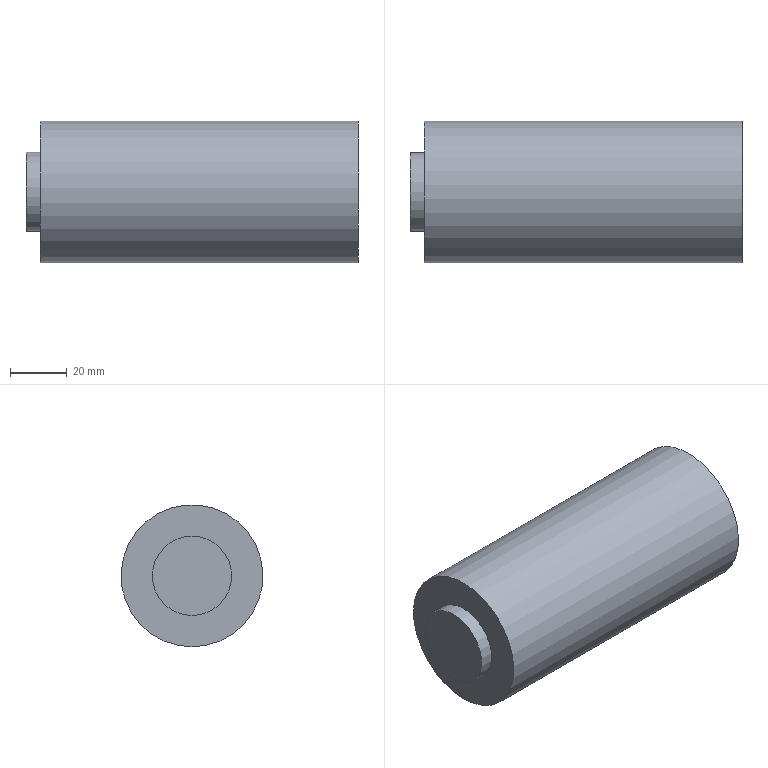Part | NX | features solid 2 | 1 solid | 5 faces | box 117 x 50 x 50 mm | volume 222990 mm3 | plane 3 | cylinder 2 | commonest cylinder face diameters 28 x1 50 x1
STEP:
#1=CARTESIAN_POINT('',(580.,930.,-200.));
#2=VERTEX_POINT('',#1);
#3=CARTESIAN_POINT('',(580.,930.,-175.));
#4=DIRECTION('',(-1.,0.,0.));
#5=DIRECTION('',(0.,0.,-1.));
#6=AXIS2_PLACEMENT_3D('',#3,#4,#5);
#7=CIRCLE('',#6,25.);
#8=EDGE_CURVE('',#2,#2,#7,.T.);
#9=ORIENTED_EDGE('',*,*,#8,.T.);
#10=EDGE_LOOP('',(#9));
#11=FACE_BOUND('',#10,.T.);
#12=CARTESIAN_POINT('',(580.,930.,-189.));
#13=VERTEX_POINT('',#12);
#14=CARTESIAN_POINT('',(580.,930.,-175.));
#15=DIRECTION('',(-1.,0.,0.));
#16=DIRECTION('',(0.,0.,-1.));
#17=AXIS2_PLACEMENT_3D('',#14,#15,#16);
#18=CIRCLE('',#17,14.);
#19=EDGE_CURVE('',#13,#13,#18,.T.);
#20=ORIENTED_EDGE('',*,*,#19,.F.);
#21=EDGE_LOOP('',(#20));
#22=FACE_BOUND('',#21,.T.);
#23=CARTESIAN_POINT('',(580.,930.,-175.));
#24=DIRECTION('',(-1.,0.,0.));
#25=DIRECTION('',(0.,0.,-1.));
#26=AXIS2_PLACEMENT_3D('',#23,#24,#25);
#27=PLANE('',#26);
#28=ADVANCED_FACE('',(#11,#22),#27,.T.);
#29=CARTESIAN_POINT('',(692.,930.,-200.));
#30=VERTEX_POINT('',#29);
#31=CARTESIAN_POINT('',(692.,930.,-175.));
#32=DIRECTION('',(1.,0.,0.));
#33=DIRECTION('',(0.,0.,-1.));
#34=AXIS2_PLACEMENT_3D('',#31,#32,#33);
#35=CIRCLE('',#34,25.);
#36=EDGE_CURVE('',#30,#30,#35,.F.);
#37=ORIENTED_EDGE('',*,*,#36,.T.);
#38=EDGE_LOOP('',(#37));
#39=FACE_BOUND('',#38,.T.);
#40=ORIENTED_EDGE('',*,*,#8,.F.);
#41=EDGE_LOOP('',(#40));
#42=FACE_BOUND('',#41,.T.);
#43=CARTESIAN_POINT('',(663.,930.,-175.));
#44=DIRECTION('',(-1.,0.,0.));
#45=DIRECTION('',(0.,0.,-1.));
#46=AXIS2_PLACEMENT_3D('',#43,#44,#45);
#47=CYLINDRICAL_SURFACE('',#46,25.);
#48=ADVANCED_FACE('',(#39,#42),#47,.T.);
#49=ORIENTED_EDGE('',*,*,#36,.F.);
#50=EDGE_LOOP('',(#49));
#51=FACE_BOUND('',#50,.T.);
#52=CARTESIAN_POINT('',(692.,905.,-175.));
#53=DIRECTION('',(1.,0.,0.));
#54=DIRECTION('',(0.,0.,1.));
#55=AXIS2_PLACEMENT_3D('',#52,#53,#54);
#56=PLANE('',#55);
#57=ADVANCED_FACE('',(#51),#56,.T.);
#58=CARTESIAN_POINT('',(575.,930.,-189.));
#59=VERTEX_POINT('',#58);
#60=CARTESIAN_POINT('',(575.,930.,-175.));
#61=DIRECTION('',(-1.,0.,0.));
#62=DIRECTION('',(0.,0.,-1.));
#63=AXIS2_PLACEMENT_3D('',#60,#61,#62);
#64=CIRCLE('',#63,14.);
#65=EDGE_CURVE('',#59,#59,#64,.T.);
#66=ORIENTED_EDGE('',*,*,#65,.F.);
#67=EDGE_LOOP('',(#66));
#68=FACE_BOUND('',#67,.T.);
#69=ORIENTED_EDGE('',*,*,#19,.T.);
#70=EDGE_LOOP('',(#69));
#71=FACE_BOUND('',#70,.T.);
#72=CARTESIAN_POINT('',(560.,930.,-175.));
#73=DIRECTION('',(1.,0.,0.));
#74=DIRECTION('',(0.,0.,1.));
#75=AXIS2_PLACEMENT_3D('',#72,#73,#74);
#76=CYLINDRICAL_SURFACE('',#75,14.);
#77=ADVANCED_FACE('',(#68,#71),#76,.T.);
#78=ORIENTED_EDGE('',*,*,#65,.T.);
#79=EDGE_LOOP('',(#78));
#80=FACE_BOUND('',#79,.T.);
#81=CARTESIAN_POINT('',(575.,930.,-175.));
#82=DIRECTION('',(-1.,0.,0.));
#83=DIRECTION('',(0.,0.,-1.));
#84=AXIS2_PLACEMENT_3D('',#81,#82,#83);
#85=PLANE('',#84);
#86=ADVANCED_FACE('',(#80),#85,.T.);
#87=CLOSED_SHELL('',(#28,#48,#57,#77,#86));
#88=MANIFOLD_SOLID_BREP('',#87);
#89=(LENGTH_UNIT()NAMED_UNIT(*)SI_UNIT(.MILLI.,.METRE.));
#90=UNCERTAINTY_MEASURE_WITH_UNIT(LENGTH_MEASURE(0.00001),#89,'','');
#91=(NAMED_UNIT(*)PLANE_ANGLE_UNIT()SI_UNIT($,.RADIAN.));
#92=(NAMED_UNIT(*)SI_UNIT($,.STERADIAN.)SOLID_ANGLE_UNIT());
#93=(GEOMETRIC_REPRESENTATION_CONTEXT(3)GLOBAL_UNCERTAINTY_ASSIGNED_CONTEXT((#90))GLOBAL_UNIT_ASSIGNED_CONTEXT((#89,#91,#92))REPRESENTATION_CONTEXT('',''));
#94=ADVANCED_BREP_SHAPE_REPRESENTATION('',(#88),#93);